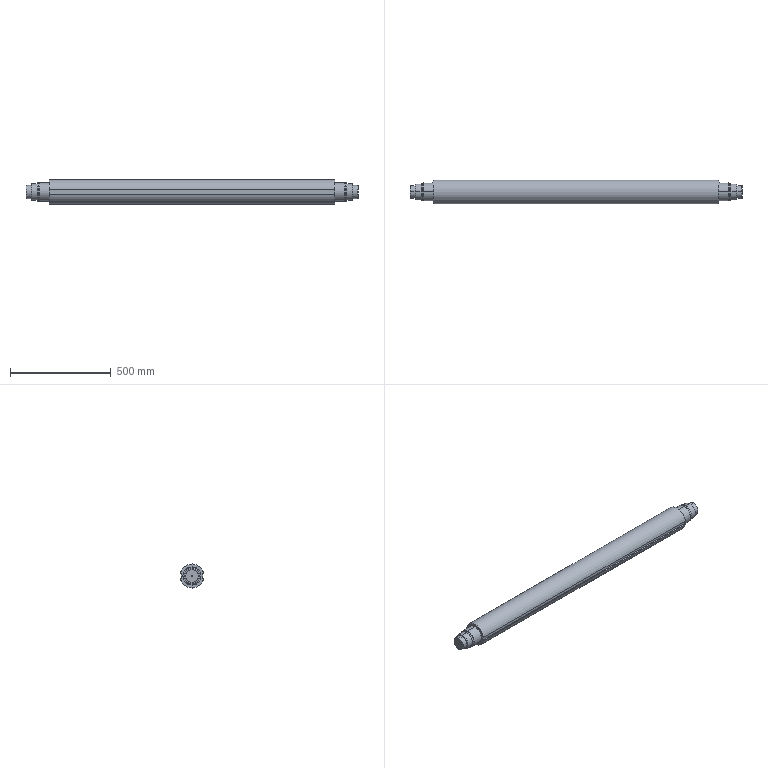Part | SolidWorks | features BaseBody 1 | 1 solid | 77 faces | box 1650 x 118.322 x 120 mm | volume 16863091 mm3 | cylinder 31 | plane 24 | cone 22 | commonest cylinder face diameters 90 x8 6 x4 20 x4 65 x4 80 x4 86 x4